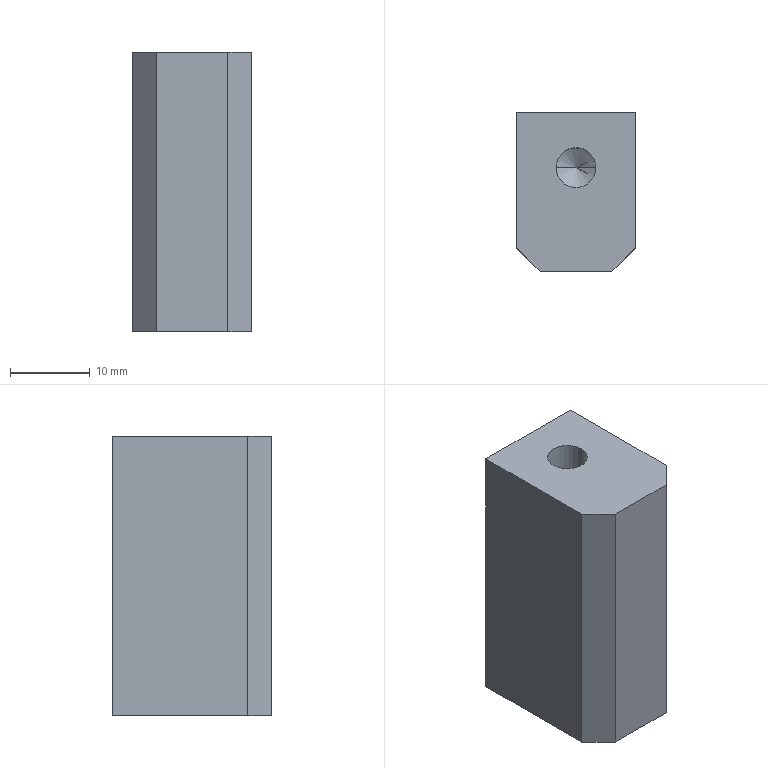Part | SolidWorks | features Chamfer 1, Extrusion 1, HoleWzd 1 | 1 solid | 12 faces | box 15 x 20 x 35 mm | volume 9881 mm3 | plane 8 | cylinder 2 | cone 2 | commonest cylinder face diameters 5 x2
STEP:
#1=CARTESIAN_POINT('',(-2.5,3.03,2.5));
#2=VERTEX_POINT('',#1);
#3=CARTESIAN_POINT('',(2.5,3.03,2.5));
#4=VERTEX_POINT('',#3);
#5=CARTESIAN_POINT('',(0.,3.03,2.5));
#6=DIRECTION('',(0.,0.,1.));
#7=DIRECTION('',(1.,0.,0.));
#8=AXIS2_PLACEMENT_3D('',#5,#6,#7);
#9=CIRCLE('',#8,2.5);
#10=EDGE_CURVE('',#2,#4,#9,.T.);
#11=ORIENTED_EDGE('',*,*,#10,.F.);
#12=CARTESIAN_POINT('',(-2.5,3.03,17.5));
#13=VERTEX_POINT('',#12);
#14=CARTESIAN_POINT('',(-2.5,3.03,17.5));
#15=DIRECTION('',(0.,0.,1.));
#16=VECTOR('',#15,1000.);
#17=LINE('',#14,#16);
#18=EDGE_CURVE('',#2,#13,#17,.T.);
#19=ORIENTED_EDGE('',*,*,#18,.T.);
#20=CARTESIAN_POINT('',(2.5,3.03,17.5));
#21=VERTEX_POINT('',#20);
#22=CARTESIAN_POINT('',(0.,3.03,17.5));
#23=DIRECTION('',(0.,0.,1.));
#24=DIRECTION('',(1.,0.,0.));
#25=AXIS2_PLACEMENT_3D('',#22,#23,#24);
#26=CIRCLE('',#25,2.5);
#27=EDGE_CURVE('',#13,#21,#26,.T.);
#28=ORIENTED_EDGE('',*,*,#27,.T.);
#29=CARTESIAN_POINT('',(2.5,3.03,17.5));
#30=DIRECTION('',(0.,0.,1.));
#31=VECTOR('',#30,1000.);
#32=LINE('',#29,#31);
#33=EDGE_CURVE('',#4,#21,#32,.T.);
#34=ORIENTED_EDGE('',*,*,#33,.F.);
#35=EDGE_LOOP('',(#11,#19,#28,#34));
#36=FACE_OUTER_BOUND('',#35,.T.);
#37=CARTESIAN_POINT('',(0.,3.03,17.5));
#38=DIRECTION('',(0.,0.,1.));
#39=DIRECTION('',(1.,0.,0.));
#40=AXIS2_PLACEMENT_3D('',#37,#38,#39);
#41=CYLINDRICAL_SURFACE('',#40,2.5);
#42=ADVANCED_FACE('',(#36),#41,.F.);
#43=CARTESIAN_POINT('',(0.,3.03,0.9978));
#44=VERTEX_POINT('',#43);
#45=CARTESIAN_POINT('',(2.5,3.03,2.5));
#46=DIRECTION('',(0.8572,0.,0.515));
#47=VECTOR('',#46,1000.);
#48=LINE('',#45,#47);
#49=EDGE_CURVE('',#44,#4,#48,.T.);
#50=ORIENTED_EDGE('',*,*,#49,.F.);
#51=CARTESIAN_POINT('',(-2.5,3.03,2.5));
#52=DIRECTION('',(-0.8572,0.,0.515));
#53=VECTOR('',#52,1000.);
#54=LINE('',#51,#53);
#55=EDGE_CURVE('',#44,#2,#54,.T.);
#56=ORIENTED_EDGE('',*,*,#55,.T.);
#57=ORIENTED_EDGE('',*,*,#10,.T.);
#58=EDGE_LOOP('',(#50,#56,#57));
#59=FACE_OUTER_BOUND('',#58,.T.);
#60=CARTESIAN_POINT('',(0.,3.03,2.5));
#61=DIRECTION('',(0.,0.,1.));
#62=DIRECTION('',(1.,0.,0.));
#63=AXIS2_PLACEMENT_3D('',#60,#61,#62);
#64=CONICAL_SURFACE('',#63,2.5,1.03);
#65=ADVANCED_FACE('',(#59),#64,.F.);
#66=CARTESIAN_POINT('',(7.5,-7.,17.5));
#67=VERTEX_POINT('',#66);
#68=CARTESIAN_POINT('',(7.5,10.,17.5));
#69=VERTEX_POINT('',#68);
#70=CARTESIAN_POINT('',(7.5,10.,17.5));
#71=DIRECTION('',(0.,1.,0.));
#72=VECTOR('',#71,1000.);
#73=LINE('',#70,#72);
#74=EDGE_CURVE('',#67,#69,#73,.T.);
#75=ORIENTED_EDGE('',*,*,#74,.F.);
#76=CARTESIAN_POINT('',(7.5,-7.,-17.5));
#77=VERTEX_POINT('',#76);
#78=CARTESIAN_POINT('',(7.5,-7.,17.5));
#79=DIRECTION('',(0.,0.,-1.));
#80=VECTOR('',#79,1000.);
#81=LINE('',#78,#80);
#82=EDGE_CURVE('',#67,#77,#81,.T.);
#83=ORIENTED_EDGE('',*,*,#82,.T.);
#84=CARTESIAN_POINT('',(7.5,10.,-17.5));
#85=VERTEX_POINT('',#84);
#86=CARTESIAN_POINT('',(7.5,10.,-17.5));
#87=DIRECTION('',(0.,1.,0.));
#88=VECTOR('',#87,1000.);
#89=LINE('',#86,#88);
#90=EDGE_CURVE('',#77,#85,#89,.T.);
#91=ORIENTED_EDGE('',*,*,#90,.T.);
#92=CARTESIAN_POINT('',(7.5,10.,17.5));
#93=DIRECTION('',(0.,0.,-1.));
#94=VECTOR('',#93,1000.);
#95=LINE('',#92,#94);
#96=EDGE_CURVE('',#69,#85,#95,.T.);
#97=ORIENTED_EDGE('',*,*,#96,.F.);
#98=EDGE_LOOP('',(#75,#83,#91,#97));
#99=FACE_OUTER_BOUND('',#98,.T.);
#100=CARTESIAN_POINT('',(7.5,10.,17.5));
#101=DIRECTION('',(-1.,0.,0.));
#102=DIRECTION('',(0.,-1.,0.));
#103=AXIS2_PLACEMENT_3D('',#100,#101,#102);
#104=PLANE('',#103);
#105=ADVANCED_FACE('',(#99),#104,.F.);
#106=CARTESIAN_POINT('',(-7.5,10.,-17.5));
#107=VERTEX_POINT('',#106);
#108=CARTESIAN_POINT('',(-7.5,10.,-17.5));
#109=DIRECTION('',(-1.,0.,0.));
#110=VECTOR('',#109,1000.);
#111=LINE('',#108,#110);
#112=EDGE_CURVE('',#85,#107,#111,.T.);
#113=ORIENTED_EDGE('',*,*,#112,.T.);
#114=CARTESIAN_POINT('',(-7.5,10.,17.5));
#115=VERTEX_POINT('',#114);
#116=CARTESIAN_POINT('',(-7.5,10.,17.5));
#117=DIRECTION('',(0.,0.,-1.));
#118=VECTOR('',#117,1000.);
#119=LINE('',#116,#118);
#120=EDGE_CURVE('',#115,#107,#119,.T.);
#121=ORIENTED_EDGE('',*,*,#120,.F.);
#122=CARTESIAN_POINT('',(-7.5,10.,17.5));
#123=DIRECTION('',(-1.,0.,0.));
#124=VECTOR('',#123,1000.);
#125=LINE('',#122,#124);
#126=EDGE_CURVE('',#69,#115,#125,.T.);
#127=ORIENTED_EDGE('',*,*,#126,.F.);
#128=ORIENTED_EDGE('',*,*,#96,.T.);
#129=EDGE_LOOP('',(#113,#121,#127,#128));
#130=FACE_OUTER_BOUND('',#129,.T.);
#131=CARTESIAN_POINT('',(-7.5,10.,17.5));
#132=DIRECTION('',(0.,-1.,0.));
#133=DIRECTION('',(1.,0.,0.));
#134=AXIS2_PLACEMENT_3D('',#131,#132,#133);
#135=PLANE('',#134);
#136=ADVANCED_FACE('',(#130),#135,.F.);
#137=CARTESIAN_POINT('',(-7.5,-7.,-17.5));
#138=VERTEX_POINT('',#137);
#139=CARTESIAN_POINT('',(-7.5,10.,-17.5));
#140=DIRECTION('',(0.,-1.,0.));
#141=VECTOR('',#140,1000.);
#142=LINE('',#139,#141);
#143=EDGE_CURVE('',#107,#138,#142,.T.);
#144=ORIENTED_EDGE('',*,*,#143,.T.);
#145=CARTESIAN_POINT('',(-7.5,-7.,17.5));
#146=VERTEX_POINT('',#145);
#147=CARTESIAN_POINT('',(-7.5,-7.,17.5));
#148=DIRECTION('',(0.,0.,1.));
#149=VECTOR('',#148,1000.);
#150=LINE('',#147,#149);
#151=EDGE_CURVE('',#138,#146,#150,.T.);
#152=ORIENTED_EDGE('',*,*,#151,.T.);
#153=CARTESIAN_POINT('',(-7.5,10.,17.5));
#154=DIRECTION('',(0.,-1.,0.));
#155=VECTOR('',#154,1000.);
#156=LINE('',#153,#155);
#157=EDGE_CURVE('',#115,#146,#156,.T.);
#158=ORIENTED_EDGE('',*,*,#157,.F.);
#159=ORIENTED_EDGE('',*,*,#120,.T.);
#160=EDGE_LOOP('',(#144,#152,#158,#159));
#161=FACE_OUTER_BOUND('',#160,.T.);
#162=CARTESIAN_POINT('',(-7.5,10.,17.5));
#163=DIRECTION('',(1.,0.,0.));
#164=DIRECTION('',(0.,1.,0.));
#165=AXIS2_PLACEMENT_3D('',#162,#163,#164);
#166=PLANE('',#165);
#167=ADVANCED_FACE('',(#161),#166,.F.);
#168=CARTESIAN_POINT('',(-4.5,-10.,-17.5));
#169=VERTEX_POINT('',#168);
#170=CARTESIAN_POINT('',(4.5,-10.,-17.5));
#171=VERTEX_POINT('',#170);
#172=CARTESIAN_POINT('',(-7.5,-10.,-17.5));
#173=DIRECTION('',(1.,0.,0.));
#174=VECTOR('',#173,1000.);
#175=LINE('',#172,#174);
#176=EDGE_CURVE('',#169,#171,#175,.T.);
#177=ORIENTED_EDGE('',*,*,#176,.T.);
#178=CARTESIAN_POINT('',(4.5,-10.,17.5));
#179=VERTEX_POINT('',#178);
#180=CARTESIAN_POINT('',(4.5,-10.,17.5));
#181=DIRECTION('',(0.,0.,1.));
#182=VECTOR('',#181,1000.);
#183=LINE('',#180,#182);
#184=EDGE_CURVE('',#171,#179,#183,.T.);
#185=ORIENTED_EDGE('',*,*,#184,.T.);
#186=CARTESIAN_POINT('',(-4.5,-10.,17.5));
#187=VERTEX_POINT('',#186);
#188=CARTESIAN_POINT('',(-7.5,-10.,17.5));
#189=DIRECTION('',(1.,0.,0.));
#190=VECTOR('',#189,1000.);
#191=LINE('',#188,#190);
#192=EDGE_CURVE('',#187,#179,#191,.T.);
#193=ORIENTED_EDGE('',*,*,#192,.F.);
#194=CARTESIAN_POINT('',(-4.5,-10.,17.5));
#195=DIRECTION('',(0.,0.,-1.));
#196=VECTOR('',#195,1000.);
#197=LINE('',#194,#196);
#198=EDGE_CURVE('',#187,#169,#197,.T.);
#199=ORIENTED_EDGE('',*,*,#198,.T.);
#200=EDGE_LOOP('',(#177,#185,#193,#199));
#201=FACE_OUTER_BOUND('',#200,.T.);
#202=CARTESIAN_POINT('',(-7.5,-10.,17.5));
#203=DIRECTION('',(0.,1.,0.));
#204=DIRECTION('',(0.,0.,1.));
#205=AXIS2_PLACEMENT_3D('',#202,#203,#204);
#206=PLANE('',#205);
#207=ADVANCED_FACE('',(#201),#206,.F.);
#208=CARTESIAN_POINT('',(0.,3.03,17.5));
#209=DIRECTION('',(0.,0.,1.));
#210=DIRECTION('',(1.,0.,0.));
#211=AXIS2_PLACEMENT_3D('',#208,#209,#210);
#212=CIRCLE('',#211,2.5);
#213=EDGE_CURVE('',#21,#13,#212,.T.);
#214=ORIENTED_EDGE('',*,*,#213,.F.);
#215=ORIENTED_EDGE('',*,*,#27,.F.);
#216=EDGE_LOOP('',(#214,#215));
#217=FACE_BOUND('',#216,.T.);
#218=ORIENTED_EDGE('',*,*,#192,.T.);
#219=CARTESIAN_POINT('',(7.25,-7.25,17.5));
#220=DIRECTION('',(0.7071,0.7071,0.));
#221=VECTOR('',#220,1000.);
#222=LINE('',#219,#221);
#223=EDGE_CURVE('',#179,#67,#222,.T.);
#224=ORIENTED_EDGE('',*,*,#223,.T.);
#225=ORIENTED_EDGE('',*,*,#74,.T.);
#226=ORIENTED_EDGE('',*,*,#126,.T.);
#227=ORIENTED_EDGE('',*,*,#157,.T.);
#228=CARTESIAN_POINT('',(-7.25,-7.25,17.5));
#229=DIRECTION('',(0.7071,-0.7071,0.));
#230=VECTOR('',#229,1000.);
#231=LINE('',#228,#230);
#232=EDGE_CURVE('',#146,#187,#231,.T.);
#233=ORIENTED_EDGE('',*,*,#232,.T.);
#234=EDGE_LOOP('',(#218,#224,#225,#226,#227,#233));
#235=FACE_OUTER_BOUND('',#234,.T.);
#236=CARTESIAN_POINT('',(0.,0.,17.5));
#237=DIRECTION('',(0.,0.,1.));
#238=DIRECTION('',(1.,0.,0.));
#239=AXIS2_PLACEMENT_3D('',#236,#237,#238);
#240=PLANE('',#239);
#241=ADVANCED_FACE('',(#217,#235),#240,.T.);
#242=ORIENTED_EDGE('',*,*,#90,.F.);
#243=CARTESIAN_POINT('',(7.5,-7.,-17.5));
#244=DIRECTION('',(-0.7071,-0.7071,0.));
#245=VECTOR('',#244,1000.);
#246=LINE('',#243,#245);
#247=EDGE_CURVE('',#77,#171,#246,.T.);
#248=ORIENTED_EDGE('',*,*,#247,.T.);
#249=ORIENTED_EDGE('',*,*,#176,.F.);
#250=CARTESIAN_POINT('',(-4.5,-10.,-17.5));
#251=DIRECTION('',(-0.7071,0.7071,0.));
#252=VECTOR('',#251,1000.);
#253=LINE('',#250,#252);
#254=EDGE_CURVE('',#169,#138,#253,.T.);
#255=ORIENTED_EDGE('',*,*,#254,.T.);
#256=ORIENTED_EDGE('',*,*,#143,.F.);
#257=ORIENTED_EDGE('',*,*,#112,.F.);
#258=EDGE_LOOP('',(#242,#248,#249,#255,#256,#257));
#259=FACE_OUTER_BOUND('',#258,.T.);
#260=CARTESIAN_POINT('',(0.,0.,-17.5));
#261=DIRECTION('',(0.,0.,1.));
#262=DIRECTION('',(1.,0.,0.));
#263=AXIS2_PLACEMENT_3D('',#260,#261,#262);
#264=PLANE('',#263);
#265=ADVANCED_FACE('',(#259),#264,.F.);
#266=ORIENTED_EDGE('',*,*,#223,.F.);
#267=ORIENTED_EDGE('',*,*,#184,.F.);
#268=ORIENTED_EDGE('',*,*,#247,.F.);
#269=ORIENTED_EDGE('',*,*,#82,.F.);
#270=EDGE_LOOP('',(#266,#267,#268,#269));
#271=FACE_OUTER_BOUND('',#270,.T.);
#272=CARTESIAN_POINT('',(7.5,-7.,17.5));
#273=DIRECTION('',(-0.7071,0.7071,0.));
#274=DIRECTION('',(0.,0.,-1.));
#275=AXIS2_PLACEMENT_3D('',#272,#273,#274);
#276=PLANE('',#275);
#277=ADVANCED_FACE('',(#271),#276,.F.);
#278=ORIENTED_EDGE('',*,*,#232,.F.);
#279=ORIENTED_EDGE('',*,*,#151,.F.);
#280=ORIENTED_EDGE('',*,*,#254,.F.);
#281=ORIENTED_EDGE('',*,*,#198,.F.);
#282=EDGE_LOOP('',(#278,#279,#280,#281));
#283=FACE_OUTER_BOUND('',#282,.T.);
#284=CARTESIAN_POINT('',(-4.5,-10.,17.5));
#285=DIRECTION('',(0.7071,0.7071,0.));
#286=DIRECTION('',(0.,0.,-1.));
#287=AXIS2_PLACEMENT_3D('',#284,#285,#286);
#288=PLANE('',#287);
#289=ADVANCED_FACE('',(#283),#288,.F.);
#290=ORIENTED_EDGE('',*,*,#55,.F.);
#291=ORIENTED_EDGE('',*,*,#49,.T.);
#292=CARTESIAN_POINT('',(0.,3.03,2.5));
#293=DIRECTION('',(0.,0.,1.));
#294=DIRECTION('',(1.,0.,0.));
#295=AXIS2_PLACEMENT_3D('',#292,#293,#294);
#296=CIRCLE('',#295,2.5);
#297=EDGE_CURVE('',#4,#2,#296,.T.);
#298=ORIENTED_EDGE('',*,*,#297,.T.);
#299=EDGE_LOOP('',(#290,#291,#298));
#300=FACE_OUTER_BOUND('',#299,.T.);
#301=CARTESIAN_POINT('',(0.,3.03,2.5));
#302=DIRECTION('',(0.,0.,1.));
#303=DIRECTION('',(1.,0.,0.));
#304=AXIS2_PLACEMENT_3D('',#301,#302,#303);
#305=CONICAL_SURFACE('',#304,2.5,1.03);
#306=ADVANCED_FACE('',(#300),#305,.F.);
#307=ORIENTED_EDGE('',*,*,#18,.F.);
#308=ORIENTED_EDGE('',*,*,#297,.F.);
#309=ORIENTED_EDGE('',*,*,#33,.T.);
#310=ORIENTED_EDGE('',*,*,#213,.T.);
#311=EDGE_LOOP('',(#307,#308,#309,#310));
#312=FACE_OUTER_BOUND('',#311,.T.);
#313=CARTESIAN_POINT('',(0.,3.03,17.5));
#314=DIRECTION('',(0.,0.,1.));
#315=DIRECTION('',(1.,0.,0.));
#316=AXIS2_PLACEMENT_3D('',#313,#314,#315);
#317=CYLINDRICAL_SURFACE('',#316,2.5);
#318=ADVANCED_FACE('',(#312),#317,.F.);
#319=CLOSED_SHELL('',(#42,#65,#105,#136,#167,#207,#241,#265,#277,#289,#306,#318));
#320=MANIFOLD_SOLID_BREP('',#319);
#321=CARTESIAN_POINT('',(0.,0.,0.));
#322=DIRECTION('',(0.,0.,1.));
#323=DIRECTION('',(1.,0.,0.));
#324=AXIS2_PLACEMENT_3D('',#321,#322,#323);
#325=(LENGTH_UNIT()NAMED_UNIT(*)SI_UNIT(.MILLI.,.METRE.));
#326=UNCERTAINTY_MEASURE_WITH_UNIT(LENGTH_MEASURE(0.00001),#325,'','');
#327=(NAMED_UNIT(*)PLANE_ANGLE_UNIT()SI_UNIT($,.RADIAN.));
#328=(NAMED_UNIT(*)SI_UNIT($,.STERADIAN.)SOLID_ANGLE_UNIT());
#329=(GEOMETRIC_REPRESENTATION_CONTEXT(3)GLOBAL_UNCERTAINTY_ASSIGNED_CONTEXT((#326))GLOBAL_UNIT_ASSIGNED_CONTEXT((#325,#327,#328))REPRESENTATION_CONTEXT('',''));
#330=ADVANCED_BREP_SHAPE_REPRESENTATION('',(#320,#324),#329);